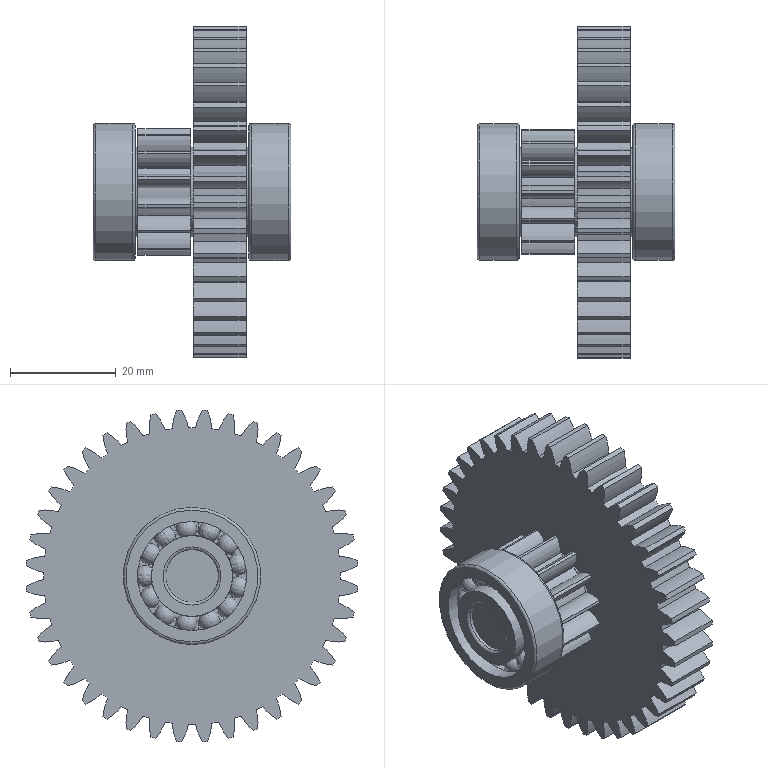Part | NX | features BREP 5 | 8 solids | 359 faces | box 37.5 x 62.872 x 62.872 mm | volume 38353 mm3 | cylinder 241 | torus 60 | plane 30 | sphere 26 | cone 2 | commonest cylinder face diameters 24 x94 56.248 x40 63 x40 8.4 x28 17.248 x14 4 x4